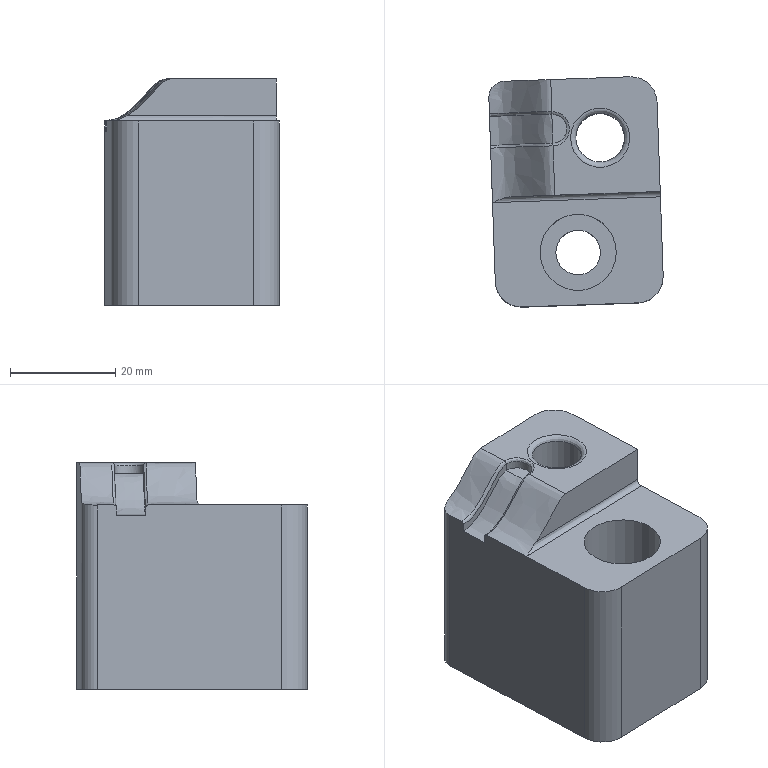Part | NX | features DIE-56 2 | 1 solid | 28 faces | box 33.153 x 43.746 x 43 mm | volume 45165 mm3 | plane 10 | spline 9 | cylinder 8 | torus 1 | commonest cylinder face diameters 10 x3 2 x1 6 x1 8.5 x1 9.27 x1 14.5 x1